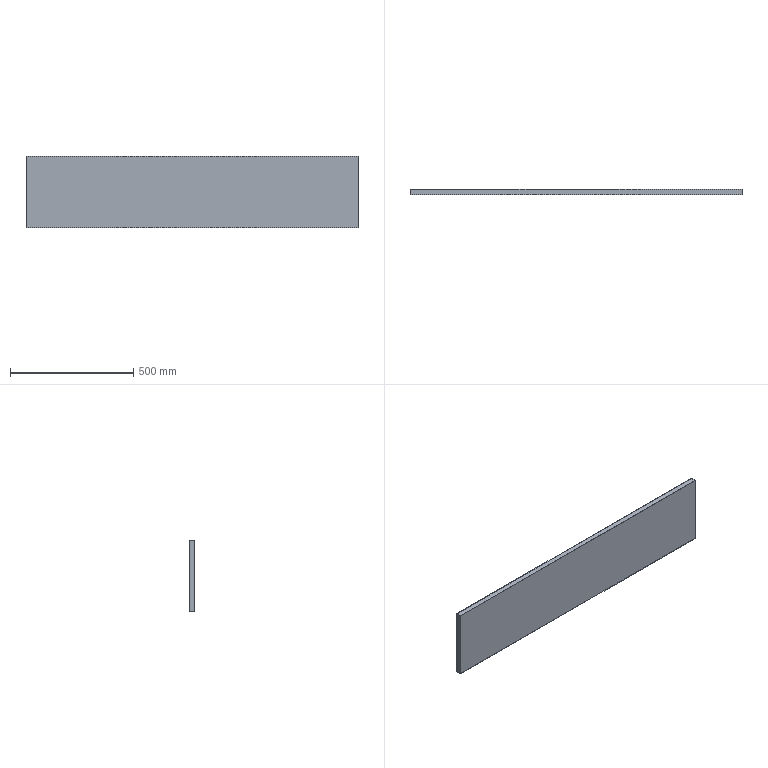Part | SolidWorks | features ICE 2, Extrusion 1, Shell 1 | 1 solid | 16 faces | box 1346 x 22 x 288 mm | volume 1655952 mm3 | plane 16
STEP:
#1=CARTESIAN_POINT('',(-671.,-20.,-142.));
#2=VERTEX_POINT('',#1);
#3=CARTESIAN_POINT('',(-671.,-20.,142.));
#4=VERTEX_POINT('',#3);
#5=CARTESIAN_POINT('',(-671.,-20.,144.));
#6=DIRECTION('',(0.,0.,1.));
#7=VECTOR('',#6,1000.);
#8=LINE('',#5,#7);
#9=EDGE_CURVE('',#2,#4,#8,.T.);
#10=ORIENTED_EDGE('',*,*,#9,.T.);
#11=CARTESIAN_POINT('',(671.,-20.,142.));
#12=VERTEX_POINT('',#11);
#13=CARTESIAN_POINT('',(-673.,-20.,142.));
#14=DIRECTION('',(1.,0.,0.));
#15=VECTOR('',#14,1000.);
#16=LINE('',#13,#15);
#17=EDGE_CURVE('',#4,#12,#16,.T.);
#18=ORIENTED_EDGE('',*,*,#17,.T.);
#19=CARTESIAN_POINT('',(671.,-20.,-142.));
#20=VERTEX_POINT('',#19);
#21=CARTESIAN_POINT('',(671.,-20.,144.));
#22=DIRECTION('',(0.,0.,-1.));
#23=VECTOR('',#22,1000.);
#24=LINE('',#21,#23);
#25=EDGE_CURVE('',#12,#20,#24,.T.);
#26=ORIENTED_EDGE('',*,*,#25,.T.);
#27=CARTESIAN_POINT('',(-673.,-20.,-142.));
#28=DIRECTION('',(-1.,0.,0.));
#29=VECTOR('',#28,1000.);
#30=LINE('',#27,#29);
#31=EDGE_CURVE('',#20,#2,#30,.T.);
#32=ORIENTED_EDGE('',*,*,#31,.T.);
#33=EDGE_LOOP('',(#10,#18,#26,#32));
#34=FACE_OUTER_BOUND('',#33,.T.);
#35=CARTESIAN_POINT('',(-673.,-20.,144.));
#36=DIRECTION('',(0.,1.,0.));
#37=DIRECTION('',(0.,0.,1.));
#38=AXIS2_PLACEMENT_3D('',#35,#36,#37);
#39=PLANE('',#38);
#40=ADVANCED_FACE('',(#34),#39,.T.);
#41=CARTESIAN_POINT('',(105.,-2.,-94.));
#42=VERTEX_POINT('',#41);
#43=CARTESIAN_POINT('',(-45.,-2.,-94.));
#44=VERTEX_POINT('',#43);
#45=CARTESIAN_POINT('',(-45.,-2.,-94.));
#46=DIRECTION('',(-1.,0.,0.));
#47=VECTOR('',#46,1000.);
#48=LINE('',#45,#47);
#49=EDGE_CURVE('',#42,#44,#48,.T.);
#50=ORIENTED_EDGE('',*,*,#49,.T.);
#51=CARTESIAN_POINT('',(-45.,-2.,-54.));
#52=VERTEX_POINT('',#51);
#53=CARTESIAN_POINT('',(-45.,-2.,-94.));
#54=DIRECTION('',(0.,0.,1.));
#55=VECTOR('',#54,1000.);
#56=LINE('',#53,#55);
#57=EDGE_CURVE('',#44,#52,#56,.T.);
#58=ORIENTED_EDGE('',*,*,#57,.T.);
#59=CARTESIAN_POINT('',(105.,-2.,-54.));
#60=VERTEX_POINT('',#59);
#61=CARTESIAN_POINT('',(-45.,-2.,-54.));
#62=DIRECTION('',(1.,0.,0.));
#63=VECTOR('',#62,1000.);
#64=LINE('',#61,#63);
#65=EDGE_CURVE('',#52,#60,#64,.T.);
#66=ORIENTED_EDGE('',*,*,#65,.T.);
#67=CARTESIAN_POINT('',(105.,-2.,-94.));
#68=DIRECTION('',(0.,0.,-1.));
#69=VECTOR('',#68,1000.);
#70=LINE('',#67,#69);
#71=EDGE_CURVE('',#60,#42,#70,.T.);
#72=ORIENTED_EDGE('',*,*,#71,.T.);
#73=EDGE_LOOP('',(#50,#58,#66,#72));
#74=FACE_BOUND('',#73,.T.);
#75=CARTESIAN_POINT('',(-671.,-2.,-142.));
#76=VERTEX_POINT('',#75);
#77=CARTESIAN_POINT('',(-671.,-2.,142.));
#78=VERTEX_POINT('',#77);
#79=CARTESIAN_POINT('',(-671.,-2.,144.));
#80=DIRECTION('',(0.,0.,1.));
#81=VECTOR('',#80,1000.);
#82=LINE('',#79,#81);
#83=EDGE_CURVE('',#76,#78,#82,.T.);
#84=ORIENTED_EDGE('',*,*,#83,.F.);
#85=CARTESIAN_POINT('',(671.,-2.,-142.));
#86=VERTEX_POINT('',#85);
#87=CARTESIAN_POINT('',(-673.,-2.,-142.));
#88=DIRECTION('',(-1.,0.,0.));
#89=VECTOR('',#88,1000.);
#90=LINE('',#87,#89);
#91=EDGE_CURVE('',#86,#76,#90,.T.);
#92=ORIENTED_EDGE('',*,*,#91,.F.);
#93=CARTESIAN_POINT('',(671.,-2.,142.));
#94=VERTEX_POINT('',#93);
#95=CARTESIAN_POINT('',(671.,-2.,144.));
#96=DIRECTION('',(0.,0.,-1.));
#97=VECTOR('',#96,1000.);
#98=LINE('',#95,#97);
#99=EDGE_CURVE('',#94,#86,#98,.T.);
#100=ORIENTED_EDGE('',*,*,#99,.F.);
#101=CARTESIAN_POINT('',(-673.,-2.,142.));
#102=DIRECTION('',(1.,0.,0.));
#103=VECTOR('',#102,1000.);
#104=LINE('',#101,#103);
#105=EDGE_CURVE('',#78,#94,#104,.T.);
#106=ORIENTED_EDGE('',*,*,#105,.F.);
#107=EDGE_LOOP('',(#84,#92,#100,#106));
#108=FACE_OUTER_BOUND('',#107,.T.);
#109=CARTESIAN_POINT('',(-673.,-2.,144.));
#110=DIRECTION('',(0.,1.,0.));
#111=DIRECTION('',(0.,0.,1.));
#112=AXIS2_PLACEMENT_3D('',#109,#110,#111);
#113=PLANE('',#112);
#114=ADVANCED_FACE('',(#74,#108),#113,.F.);
#115=ORIENTED_EDGE('',*,*,#105,.T.);
#116=CARTESIAN_POINT('',(671.,-20.,142.));
#117=DIRECTION('',(0.,1.,0.));
#118=VECTOR('',#117,1000.);
#119=LINE('',#116,#118);
#120=EDGE_CURVE('',#12,#94,#119,.T.);
#121=ORIENTED_EDGE('',*,*,#120,.F.);
#122=ORIENTED_EDGE('',*,*,#17,.F.);
#123=CARTESIAN_POINT('',(-671.,-20.,142.));
#124=DIRECTION('',(0.,1.,0.));
#125=VECTOR('',#124,1000.);
#126=LINE('',#123,#125);
#127=EDGE_CURVE('',#4,#78,#126,.T.);
#128=ORIENTED_EDGE('',*,*,#127,.T.);
#129=EDGE_LOOP('',(#115,#121,#122,#128));
#130=FACE_OUTER_BOUND('',#129,.T.);
#131=CARTESIAN_POINT('',(-673.,-20.,142.));
#132=DIRECTION('',(0.,0.,1.));
#133=DIRECTION('',(1.,0.,0.));
#134=AXIS2_PLACEMENT_3D('',#131,#132,#133);
#135=PLANE('',#134);
#136=ADVANCED_FACE('',(#130),#135,.F.);
#137=ORIENTED_EDGE('',*,*,#99,.T.);
#138=CARTESIAN_POINT('',(671.,-20.,-142.));
#139=DIRECTION('',(0.,1.,0.));
#140=VECTOR('',#139,1000.);
#141=LINE('',#138,#140);
#142=EDGE_CURVE('',#20,#86,#141,.T.);
#143=ORIENTED_EDGE('',*,*,#142,.F.);
#144=ORIENTED_EDGE('',*,*,#25,.F.);
#145=ORIENTED_EDGE('',*,*,#120,.T.);
#146=EDGE_LOOP('',(#137,#143,#144,#145));
#147=FACE_OUTER_BOUND('',#146,.T.);
#148=CARTESIAN_POINT('',(671.,-20.,-144.));
#149=DIRECTION('',(1.,0.,0.));
#150=DIRECTION('',(0.,0.,-1.));
#151=AXIS2_PLACEMENT_3D('',#148,#149,#150);
#152=PLANE('',#151);
#153=ADVANCED_FACE('',(#147),#152,.F.);
#154=ORIENTED_EDGE('',*,*,#91,.T.);
#155=CARTESIAN_POINT('',(-671.,-20.,-142.));
#156=DIRECTION('',(0.,1.,0.));
#157=VECTOR('',#156,1000.);
#158=LINE('',#155,#157);
#159=EDGE_CURVE('',#2,#76,#158,.T.);
#160=ORIENTED_EDGE('',*,*,#159,.F.);
#161=ORIENTED_EDGE('',*,*,#31,.F.);
#162=ORIENTED_EDGE('',*,*,#142,.T.);
#163=EDGE_LOOP('',(#154,#160,#161,#162));
#164=FACE_OUTER_BOUND('',#163,.T.);
#165=CARTESIAN_POINT('',(-673.,-20.,-142.));
#166=DIRECTION('',(0.,0.,-1.));
#167=DIRECTION('',(-1.,0.,0.));
#168=AXIS2_PLACEMENT_3D('',#165,#166,#167);
#169=PLANE('',#168);
#170=ADVANCED_FACE('',(#164),#169,.F.);
#171=ORIENTED_EDGE('',*,*,#83,.T.);
#172=ORIENTED_EDGE('',*,*,#127,.F.);
#173=ORIENTED_EDGE('',*,*,#9,.F.);
#174=ORIENTED_EDGE('',*,*,#159,.T.);
#175=EDGE_LOOP('',(#171,#172,#173,#174));
#176=FACE_OUTER_BOUND('',#175,.T.);
#177=CARTESIAN_POINT('',(-671.,-20.,-144.));
#178=DIRECTION('',(-1.,0.,0.));
#179=DIRECTION('',(0.,0.,1.));
#180=AXIS2_PLACEMENT_3D('',#177,#178,#179);
#181=PLANE('',#180);
#182=ADVANCED_FACE('',(#176),#181,.F.);
#183=CARTESIAN_POINT('',(-45.,0.,-94.));
#184=VERTEX_POINT('',#183);
#185=CARTESIAN_POINT('',(-45.,0.,-54.));
#186=VERTEX_POINT('',#185);
#187=CARTESIAN_POINT('',(-45.,0.,-94.));
#188=DIRECTION('',(0.,0.,1.));
#189=VECTOR('',#188,1000.);
#190=LINE('',#187,#189);
#191=EDGE_CURVE('',#184,#186,#190,.T.);
#192=ORIENTED_EDGE('',*,*,#191,.T.);
#193=CARTESIAN_POINT('',(-45.,-2.,-54.));
#194=DIRECTION('',(0.,1.,0.));
#195=VECTOR('',#194,1000.);
#196=LINE('',#193,#195);
#197=EDGE_CURVE('',#52,#186,#196,.T.);
#198=ORIENTED_EDGE('',*,*,#197,.F.);
#199=ORIENTED_EDGE('',*,*,#57,.F.);
#200=CARTESIAN_POINT('',(-45.,-2.,-94.));
#201=DIRECTION('',(0.,1.,0.));
#202=VECTOR('',#201,1000.);
#203=LINE('',#200,#202);
#204=EDGE_CURVE('',#44,#184,#203,.T.);
#205=ORIENTED_EDGE('',*,*,#204,.T.);
#206=EDGE_LOOP('',(#192,#198,#199,#205));
#207=FACE_OUTER_BOUND('',#206,.T.);
#208=CARTESIAN_POINT('',(-45.,-2.,-94.));
#209=DIRECTION('',(-1.,0.,0.));
#210=DIRECTION('',(0.,0.,1.));
#211=AXIS2_PLACEMENT_3D('',#208,#209,#210);
#212=PLANE('',#211);
#213=ADVANCED_FACE('',(#207),#212,.F.);
#214=CARTESIAN_POINT('',(105.,0.,-94.));
#215=VERTEX_POINT('',#214);
#216=CARTESIAN_POINT('',(-45.,0.,-94.));
#217=DIRECTION('',(-1.,0.,0.));
#218=VECTOR('',#217,1000.);
#219=LINE('',#216,#218);
#220=EDGE_CURVE('',#215,#184,#219,.T.);
#221=ORIENTED_EDGE('',*,*,#220,.T.);
#222=ORIENTED_EDGE('',*,*,#204,.F.);
#223=ORIENTED_EDGE('',*,*,#49,.F.);
#224=CARTESIAN_POINT('',(105.,-2.,-94.));
#225=DIRECTION('',(0.,1.,0.));
#226=VECTOR('',#225,1000.);
#227=LINE('',#224,#226);
#228=EDGE_CURVE('',#42,#215,#227,.T.);
#229=ORIENTED_EDGE('',*,*,#228,.T.);
#230=EDGE_LOOP('',(#221,#222,#223,#229));
#231=FACE_OUTER_BOUND('',#230,.T.);
#232=CARTESIAN_POINT('',(-45.,-2.,-94.));
#233=DIRECTION('',(0.,0.,-1.));
#234=DIRECTION('',(-1.,0.,0.));
#235=AXIS2_PLACEMENT_3D('',#232,#233,#234);
#236=PLANE('',#235);
#237=ADVANCED_FACE('',(#231),#236,.F.);
#238=CARTESIAN_POINT('',(105.,0.,-54.));
#239=VERTEX_POINT('',#238);
#240=CARTESIAN_POINT('',(105.,0.,-94.));
#241=DIRECTION('',(0.,0.,-1.));
#242=VECTOR('',#241,1000.);
#243=LINE('',#240,#242);
#244=EDGE_CURVE('',#239,#215,#243,.T.);
#245=ORIENTED_EDGE('',*,*,#244,.T.);
#246=ORIENTED_EDGE('',*,*,#228,.F.);
#247=ORIENTED_EDGE('',*,*,#71,.F.);
#248=CARTESIAN_POINT('',(105.,-2.,-54.));
#249=DIRECTION('',(0.,1.,0.));
#250=VECTOR('',#249,1000.);
#251=LINE('',#248,#250);
#252=EDGE_CURVE('',#60,#239,#251,.T.);
#253=ORIENTED_EDGE('',*,*,#252,.T.);
#254=EDGE_LOOP('',(#245,#246,#247,#253));
#255=FACE_OUTER_BOUND('',#254,.T.);
#256=CARTESIAN_POINT('',(105.,-2.,-94.));
#257=DIRECTION('',(1.,0.,0.));
#258=DIRECTION('',(0.,0.,-1.));
#259=AXIS2_PLACEMENT_3D('',#256,#257,#258);
#260=PLANE('',#259);
#261=ADVANCED_FACE('',(#255),#260,.F.);
#262=CARTESIAN_POINT('',(-45.,0.,-54.));
#263=DIRECTION('',(1.,0.,0.));
#264=VECTOR('',#263,1000.);
#265=LINE('',#262,#264);
#266=EDGE_CURVE('',#186,#239,#265,.T.);
#267=ORIENTED_EDGE('',*,*,#266,.T.);
#268=ORIENTED_EDGE('',*,*,#252,.F.);
#269=ORIENTED_EDGE('',*,*,#65,.F.);
#270=ORIENTED_EDGE('',*,*,#197,.T.);
#271=EDGE_LOOP('',(#267,#268,#269,#270));
#272=FACE_OUTER_BOUND('',#271,.T.);
#273=CARTESIAN_POINT('',(-45.,-2.,-54.));
#274=DIRECTION('',(0.,0.,1.));
#275=DIRECTION('',(1.,0.,0.));
#276=AXIS2_PLACEMENT_3D('',#273,#274,#275);
#277=PLANE('',#276);
#278=ADVANCED_FACE('',(#272),#277,.F.);
#279=CARTESIAN_POINT('',(-673.,0.,-144.));
#280=VERTEX_POINT('',#279);
#281=CARTESIAN_POINT('',(-673.,0.,144.));
#282=VERTEX_POINT('',#281);
#283=CARTESIAN_POINT('',(-673.,0.,-144.));
#284=DIRECTION('',(0.,0.,1.));
#285=VECTOR('',#284,1000.);
#286=LINE('',#283,#285);
#287=EDGE_CURVE('',#280,#282,#286,.T.);
#288=ORIENTED_EDGE('',*,*,#287,.F.);
#289=CARTESIAN_POINT('',(-673.,-22.,-144.));
#290=VERTEX_POINT('',#289);
#291=CARTESIAN_POINT('',(-673.,-20.,-144.));
#292=DIRECTION('',(0.,1.,0.));
#293=VECTOR('',#292,1000.);
#294=LINE('',#291,#293);
#295=EDGE_CURVE('',#290,#280,#294,.T.);
#296=ORIENTED_EDGE('',*,*,#295,.F.);
#297=CARTESIAN_POINT('',(-673.,-22.,144.));
#298=VERTEX_POINT('',#297);
#299=CARTESIAN_POINT('',(-673.,-22.,-144.));
#300=DIRECTION('',(0.,0.,-1.));
#301=VECTOR('',#300,1000.);
#302=LINE('',#299,#301);
#303=EDGE_CURVE('',#298,#290,#302,.T.);
#304=ORIENTED_EDGE('',*,*,#303,.F.);
#305=CARTESIAN_POINT('',(-673.,-20.,144.));
#306=DIRECTION('',(0.,1.,0.));
#307=VECTOR('',#306,1000.);
#308=LINE('',#305,#307);
#309=EDGE_CURVE('',#298,#282,#308,.T.);
#310=ORIENTED_EDGE('',*,*,#309,.T.);
#311=EDGE_LOOP('',(#288,#296,#304,#310));
#312=FACE_OUTER_BOUND('',#311,.T.);
#313=CARTESIAN_POINT('',(-673.,-20.,-144.));
#314=DIRECTION('',(-1.,0.,0.));
#315=DIRECTION('',(0.,0.,1.));
#316=AXIS2_PLACEMENT_3D('',#313,#314,#315);
#317=PLANE('',#316);
#318=ADVANCED_FACE('',(#312),#317,.T.);
#319=CARTESIAN_POINT('',(673.,0.,-144.));
#320=VERTEX_POINT('',#319);
#321=CARTESIAN_POINT('',(-673.,0.,-144.));
#322=DIRECTION('',(-1.,0.,0.));
#323=VECTOR('',#322,1000.);
#324=LINE('',#321,#323);
#325=EDGE_CURVE('',#320,#280,#324,.T.);
#326=ORIENTED_EDGE('',*,*,#325,.F.);
#327=CARTESIAN_POINT('',(673.,-22.,-144.));
#328=VERTEX_POINT('',#327);
#329=CARTESIAN_POINT('',(673.,-20.,-144.));
#330=DIRECTION('',(0.,1.,0.));
#331=VECTOR('',#330,1000.);
#332=LINE('',#329,#331);
#333=EDGE_CURVE('',#328,#320,#332,.T.);
#334=ORIENTED_EDGE('',*,*,#333,.F.);
#335=CARTESIAN_POINT('',(-673.,-22.,-144.));
#336=DIRECTION('',(1.,0.,0.));
#337=VECTOR('',#336,1000.);
#338=LINE('',#335,#337);
#339=EDGE_CURVE('',#290,#328,#338,.T.);
#340=ORIENTED_EDGE('',*,*,#339,.F.);
#341=ORIENTED_EDGE('',*,*,#295,.T.);
#342=EDGE_LOOP('',(#326,#334,#340,#341));
#343=FACE_OUTER_BOUND('',#342,.T.);
#344=CARTESIAN_POINT('',(-673.,-20.,-144.));
#345=DIRECTION('',(0.,0.,-1.));
#346=DIRECTION('',(-1.,0.,0.));
#347=AXIS2_PLACEMENT_3D('',#344,#345,#346);
#348=PLANE('',#347);
#349=ADVANCED_FACE('',(#343),#348,.T.);
#350=CARTESIAN_POINT('',(673.,0.,144.));
#351=VERTEX_POINT('',#350);
#352=CARTESIAN_POINT('',(673.,0.,-144.));
#353=DIRECTION('',(0.,0.,-1.));
#354=VECTOR('',#353,1000.);
#355=LINE('',#352,#354);
#356=EDGE_CURVE('',#351,#320,#355,.T.);
#357=ORIENTED_EDGE('',*,*,#356,.F.);
#358=CARTESIAN_POINT('',(673.,-22.,144.));
#359=VERTEX_POINT('',#358);
#360=CARTESIAN_POINT('',(673.,-20.,144.));
#361=DIRECTION('',(0.,1.,0.));
#362=VECTOR('',#361,1000.);
#363=LINE('',#360,#362);
#364=EDGE_CURVE('',#359,#351,#363,.T.);
#365=ORIENTED_EDGE('',*,*,#364,.F.);
#366=CARTESIAN_POINT('',(673.,-22.,-144.));
#367=DIRECTION('',(0.,0.,1.));
#368=VECTOR('',#367,1000.);
#369=LINE('',#366,#368);
#370=EDGE_CURVE('',#328,#359,#369,.T.);
#371=ORIENTED_EDGE('',*,*,#370,.F.);
#372=ORIENTED_EDGE('',*,*,#333,.T.);
#373=EDGE_LOOP('',(#357,#365,#371,#372));
#374=FACE_OUTER_BOUND('',#373,.T.);
#375=CARTESIAN_POINT('',(673.,-20.,-144.));
#376=DIRECTION('',(1.,0.,0.));
#377=DIRECTION('',(0.,0.,-1.));
#378=AXIS2_PLACEMENT_3D('',#375,#376,#377);
#379=PLANE('',#378);
#380=ADVANCED_FACE('',(#374),#379,.T.);
#381=CARTESIAN_POINT('',(-673.,0.,144.));
#382=DIRECTION('',(1.,0.,0.));
#383=VECTOR('',#382,1000.);
#384=LINE('',#381,#383);
#385=EDGE_CURVE('',#282,#351,#384,.T.);
#386=ORIENTED_EDGE('',*,*,#385,.F.);
#387=ORIENTED_EDGE('',*,*,#309,.F.);
#388=CARTESIAN_POINT('',(-673.,-22.,144.));
#389=DIRECTION('',(-1.,0.,0.));
#390=VECTOR('',#389,1000.);
#391=LINE('',#388,#390);
#392=EDGE_CURVE('',#359,#298,#391,.T.);
#393=ORIENTED_EDGE('',*,*,#392,.F.);
#394=ORIENTED_EDGE('',*,*,#364,.T.);
#395=EDGE_LOOP('',(#386,#387,#393,#394));
#396=FACE_OUTER_BOUND('',#395,.T.);
#397=CARTESIAN_POINT('',(-673.,-20.,144.));
#398=DIRECTION('',(0.,0.,1.));
#399=DIRECTION('',(1.,0.,0.));
#400=AXIS2_PLACEMENT_3D('',#397,#398,#399);
#401=PLANE('',#400);
#402=ADVANCED_FACE('',(#396),#401,.T.);
#403=ORIENTED_EDGE('',*,*,#191,.F.);
#404=ORIENTED_EDGE('',*,*,#220,.F.);
#405=ORIENTED_EDGE('',*,*,#244,.F.);
#406=ORIENTED_EDGE('',*,*,#266,.F.);
#407=EDGE_LOOP('',(#403,#404,#405,#406));
#408=FACE_BOUND('',#407,.T.);
#409=ORIENTED_EDGE('',*,*,#287,.T.);
#410=ORIENTED_EDGE('',*,*,#385,.T.);
#411=ORIENTED_EDGE('',*,*,#356,.T.);
#412=ORIENTED_EDGE('',*,*,#325,.T.);
#413=EDGE_LOOP('',(#409,#410,#411,#412));
#414=FACE_OUTER_BOUND('',#413,.T.);
#415=CARTESIAN_POINT('',(-673.,0.,144.));
#416=DIRECTION('',(0.,1.,0.));
#417=DIRECTION('',(0.,0.,1.));
#418=AXIS2_PLACEMENT_3D('',#415,#416,#417);
#419=PLANE('',#418);
#420=ADVANCED_FACE('',(#408,#414),#419,.T.);
#421=ORIENTED_EDGE('',*,*,#303,.T.);
#422=ORIENTED_EDGE('',*,*,#339,.T.);
#423=ORIENTED_EDGE('',*,*,#370,.T.);
#424=ORIENTED_EDGE('',*,*,#392,.T.);
#425=EDGE_LOOP('',(#421,#422,#423,#424));
#426=FACE_OUTER_BOUND('',#425,.T.);
#427=CARTESIAN_POINT('',(-673.,-22.,144.));
#428=DIRECTION('',(0.,1.,0.));
#429=DIRECTION('',(0.,0.,1.));
#430=AXIS2_PLACEMENT_3D('',#427,#428,#429);
#431=PLANE('',#430);
#432=ADVANCED_FACE('',(#426),#431,.F.);
#433=CLOSED_SHELL('',(#40,#114,#136,#153,#170,#182,#213,#237,#261,#278,#318,#349,#380,#402,#420,#432));
#434=MANIFOLD_SOLID_BREP('',#433);
#435=CARTESIAN_POINT('',(0.,0.,0.));
#436=DIRECTION('',(0.,0.,1.));
#437=DIRECTION('',(1.,0.,0.));
#438=AXIS2_PLACEMENT_3D('',#435,#436,#437);
#439=(LENGTH_UNIT()NAMED_UNIT(*)SI_UNIT(.MILLI.,.METRE.));
#440=UNCERTAINTY_MEASURE_WITH_UNIT(LENGTH_MEASURE(0.00001),#439,'','');
#441=(NAMED_UNIT(*)PLANE_ANGLE_UNIT()SI_UNIT($,.RADIAN.));
#442=(NAMED_UNIT(*)SI_UNIT($,.STERADIAN.)SOLID_ANGLE_UNIT());
#443=(GEOMETRIC_REPRESENTATION_CONTEXT(3)GLOBAL_UNCERTAINTY_ASSIGNED_CONTEXT((#440))GLOBAL_UNIT_ASSIGNED_CONTEXT((#439,#441,#442))REPRESENTATION_CONTEXT('',''));
#444=ADVANCED_BREP_SHAPE_REPRESENTATION('',(#434,#438),#443);